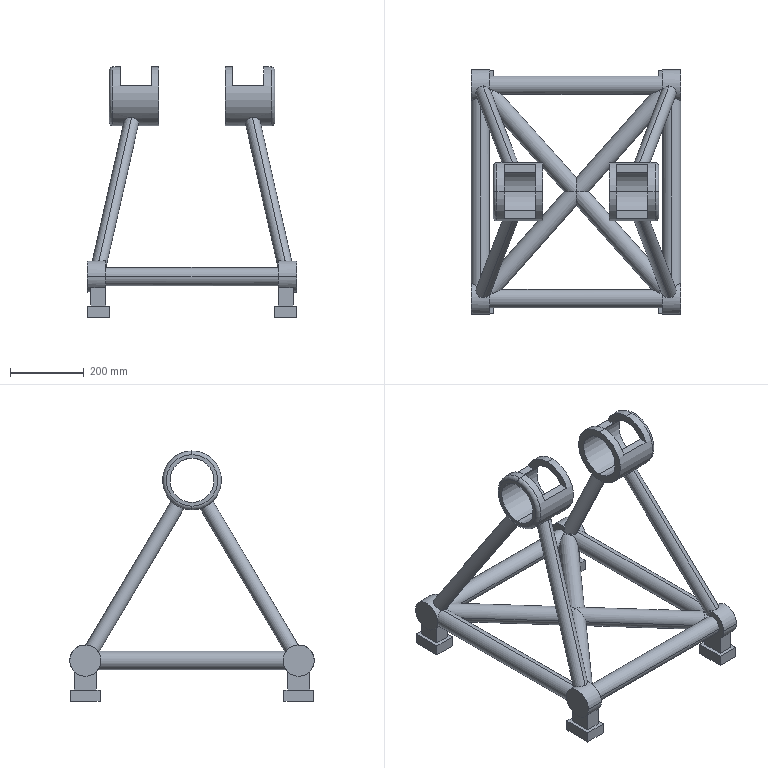Part | SolidWorks | features ICE 6, Cut 3, Sweep 3, 3DProfileFeature 2, MirrorPattern 2, Extrusion 1, Fillet 1 | 1 solid | 122 faces | box 570 x 664.853 x 679.884 mm | volume 12658453 mm3 | plane 64 | cylinder 54 | torus 4 | commonest cylinder face diameters 50 x26 84.853 x12 40 x8 120 x4 160 x4